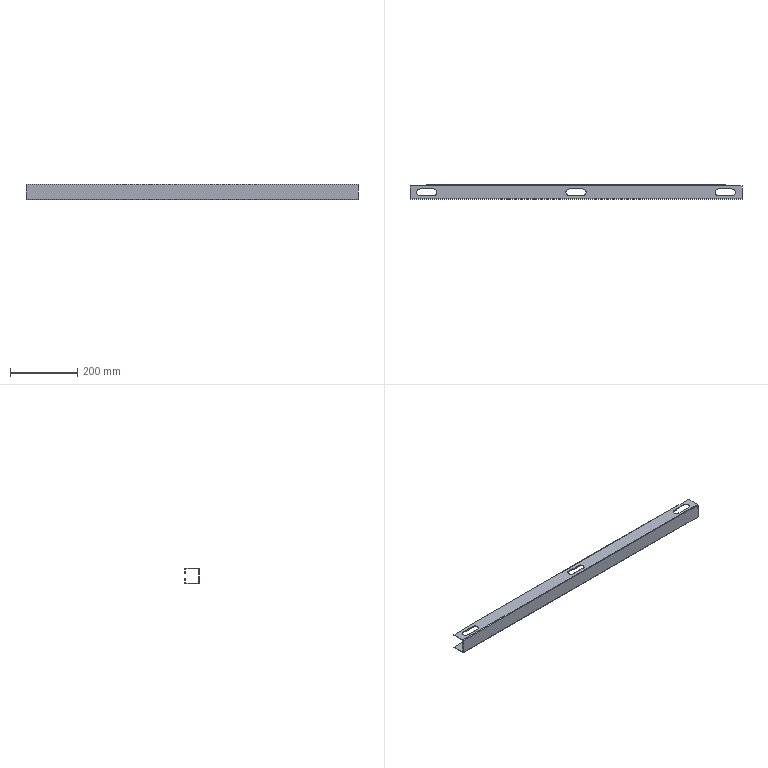Part | 1 solid | 70 faces | box 985 x 42 x 46 mm | volume 210270 mm3 | plane 50 | cylinder 20 | commonest cylinder face diameters 20 x12 0.4 x4 3.4 x4